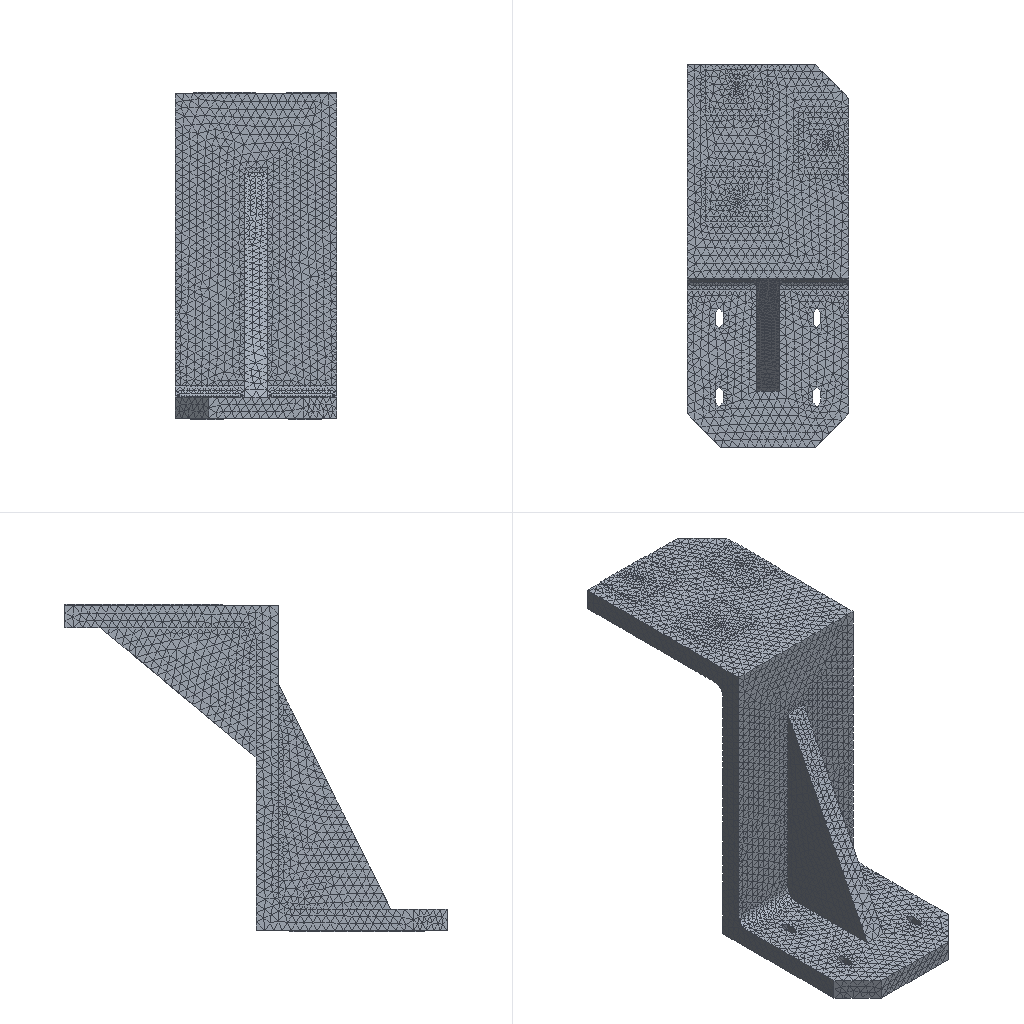Simulation study | nx simcenter
Set-up summary:
category,name,step,type,value,unit,region
solver,nx_nastran (Simcenter)
units,not stated in the deck,,not stated
analysis,deck,,static,static
analysis,solution,,SOL,101
load_step,SUBCASE 1,1,SUBCASE,SPC=1 LOAD=2
load_step,requested,,,1
mesh,nodes,,,57778
mesh,elements,,,34527
element_type,CTETRA,,solid,34527
load,nodal force total,,FX,0.0,model units
load,nodal force total,,FY,0.0,model units
load,nodal force total,,FZ,-4999999.917,model units
load,load commands in deck,,count,942
bc,support commands in deck,,count,1082
analysis,NX solution 0,,Structural,Linear Statics - Single Constraint
check,setup vs results,,match,every grid point's frame and coordinates and every element id; grid points of CTETRA elements
Nastran input file, long lists of numbers shortened:
$*$$$$$$$$$$$$$$$$$$$$$$$$$$$$$$$$$$$$$$$$$$$$$$$$$$$$$$$$$$$$$$$$$
$*
$*                    NX v10.0.0.24 TRANSLATOR
$*                    FOR NX NASTRAN VERSION 10.0
$ (33 more lines like these left out)
ASSIGN OUTPUT2='110_sim1-solution_1.op2' UNIT=12
$*
$*$$$$$$$$$$$$$$$$$$$$$$$$$$$$$$$$$$$
$*
$* EXECUTIVE CONTROL
$*
$*$$$$$$$$$$$$$$$$$$$$$$$$$$$$$$$$$$$
$*
ID,NASTRAN,110_sim1-solution_1
SOL 101
CEND
$*
$*$$$$$$$$$$$$$$$$$$$$$$$$$$$$$$$$$$$
$*
$* CASE CONTROL
$*
$*$$$$$$$$$$$$$$$$$$$$$$$$$$$$$$$$$$$
$*
TITLE = Solution 1
ECHO = NONE
SPC = 1
OUTPUT
BCRESULTS(TRACTION,FORCE,PLOT) = ALL
DISPLACEMENT(PLOT) = ALL
ESE(PLOT) = ALL
FORCE(PLOT,CORNER) = ALL
OLOAD(PLOT) = ALL
SPCFORCES(PLOT) = ALL
STRAIN(PLOT,FIBER,CORNER) = ALL
STRESS(PLOT,CORNER) = ALL
$*  NX Step: Subcase - Static Loads 1
SUBCASE 1
LABEL = Subcase - Static Loads 1
LOAD = 2
$*
$*$$$$$$$$$$$$$$$$$$$$$$$$$$$$$$$$$$$
$*
$* BULK DATA
$*
$*$$$$$$$$$$$$$$$$$$$$$$$$$$$$$$$$$$$
$*
BEGIN BULK
$*
$* PARAM CARDS
$*
PARAM      K6ROT100.0000
PARAM     OIBULK     YES
PARAM    OMACHPR     YES
PARAM       POST      -2
PARAM    POSTEXT     YES
PARAM    UNITSYS   MN-MM
$*
$* GRID CARDS
$*
GRID*              57659               00.0000000000E+00-1.900000000E+02+
*       1.0000000000E+00               0
GRID*              57660               0-1.040834086E-14-1.900000000E+02+
*       2.0000000000E+01               0
$ (115552 more lines like these left out)
$*
$* ELEMENT CARDS
$*
$*  NX Mesh Collector: Solid(1)
$*  NX Mesh: 3d_mesh(1)
CTETRA         1       1       1       2       3       4    2973    2974+
+           2975    2976    2977    2978
CTETRA         2       1       5       2       6       7    2979    2980+
+           2981    2982    2983    2984
$ (69050 more lines like these left out)
$*
$* PROPERTY CARDS
$*
$*  NX Property: PSOLID1
PSOLID         1       1       0                           SMECH
$*
$* MATERIAL CARDS
$*
$*  NX Material: Steel
MAT1           12.0694+8        0.2880007.8290-61.1141-5
MATT1          1       1               2               3
TABLEM1        1                                                        +
+        20.00002.0694+8 21.11002.0694+8    ENDT
TABLEM1        2                                                        +
+        20.00000.288000 21.11000.288000 23.89000.288000 37.78000.288000+
+        51.67000.289000 65.56000.289000 79.44000.290000 93.33000.290000+
+       107.22000.291000121.11000.291000135.00000.291000148.89000.292000+
+       162.78000.292000176.67000.293000190.56000.293000204.44000.293000+
+       218.33000.294000232.22000.294000246.11000.294000260.00000.295000+
+       273.89000.295000287.78000.296000301.67000.296000315.56000.296000+
+       329.44000.297000343.33000.297000357.22000.298000371.11000.298000+
+       385.00000.298000398.89000.299000412.78000.299000426.67000.300000+
+       440.56000.300000454.44000.301000468.33000.301000482.22000.302000+
+       496.11000.302000510.00000.303000523.89000.304000537.78000.304000+
+       551.67000.305000565.56000.306000579.44000.307000593.33000.308000+
+       607.22000.309000621.11000.310000635.00000.311000648.89000.312000+
+       662.78000.313000676.67000.314000690.56000.316000704.44000.317000+
+           ENDT
TABLEM1        3                                                        +
+        20.00001.1280-5 93.33001.1790-5107.22001.1880-5121.11001.1970-5+
+       135.00001.2060-5148.89001.2132-5162.78001.2222-5176.67001.2312-5+
+       190.56001.2402-5204.44001.2492-5218.33001.2582-5232.22001.2672-5+
+       246.11001.2762-5260.00001.2852-5273.89001.2942-5287.78001.3032-5+
+       301.67001.3122-5315.56001.3212-5329.44001.3302-5343.33001.3392-5+
+       357.22001.3464-5371.11001.3554-5385.00001.3644-5398.89001.3734-5+
+       412.78001.3806-5426.67001.3896-5440.56001.3986-5454.44001.4058-5+
+       468.33001.4148-5482.22001.4238-5496.11001.4310-5510.00001.4400-5+
+       523.89001.4472-5537.78001.4544-5551.67001.4616-5565.56001.4688-5+
+       579.44001.4742-5593.33001.4796-5607.22001.4832-5621.11001.4886-5+
+       635.00001.4904-5648.89001.4922-5662.78001.4922-5676.67001.4922-5+
+       690.56001.4904-5704.44001.4886-5718.33001.4850-5732.22001.4796-5+
+       746.11001.4724-5760.00001.4634-5773.89001.4472-5787.78001.4256-5+
+       801.67001.4004-5815.56001.3680-5    ENDT
$*
$* LOAD AND CONSTRAINT CARDS
$*
$*  NX Load and Constraint: Fixed(1)
SPC            1   35700  123456  0.0000
SPC            1   35701  123456  0.0000
SPC            1   35702  123456  0.0000
SPC            1   35703  123456  0.0000
$ (1078 more lines like these left out)
$*  NX Load and Constraint: Force(1)
FORCE          2   36639       0 4306.80  0.0000  0.0000-1.00000
FORCE          2   36640       0 4617.01  0.0000  0.0000-1.00000
FORCE          2   36641       0 5629.28  0.0000  0.0000-1.00000
FORCE          2   36642       0 3557.62  0.0000  0.0000-1.00000
$ (938 more lines like these left out)
ENDDATA 708599c7
Results summary:
result,analysis,,,static
result,last_loadstep,,,1
result,primary field,,,displacements
result,max displacement,,,0.2333,model units
result,reaction total,,FX,0.2688,model units
result,reaction total,,FY,1.151,model units
result,reaction total,,FZ,5000005.0,model units
result,NX solution 0,,loadcases,1,mm